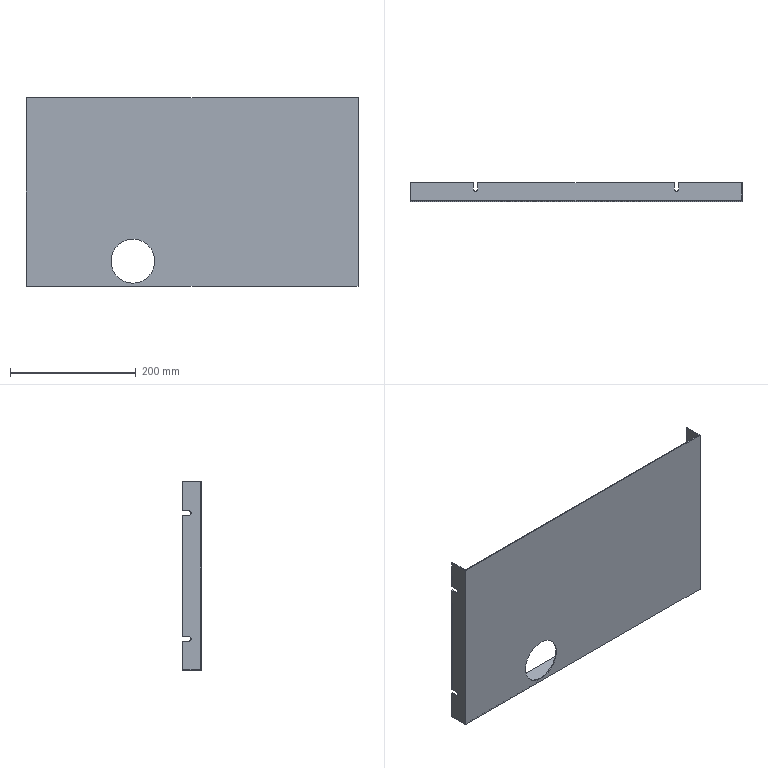Part | SolidWorks | features BaseBody 1 | 1 solid | 36 faces | box 528 x 30 x 300 mm | volume 279118 mm3 | plane 28 | cylinder 8 | commonest cylinder face diameters 7 x6 70 x2
STEP:
#1=CARTESIAN_POINT('',(-94.,1.5,-145.));
#2=VERTEX_POINT('',#1);
#3=CARTESIAN_POINT('',(-94.,1.5,-75.));
#4=VERTEX_POINT('',#3);
#5=CARTESIAN_POINT('',(-94.,1.5,-110.));
#6=DIRECTION('',(0.,1.,0.));
#7=DIRECTION('',(0.,0.,-1.));
#8=AXIS2_PLACEMENT_3D('',#5,#6,#7);
#9=CIRCLE('',#8,35.);
#10=EDGE_CURVE('',#2,#4,#9,.T.);
#11=ORIENTED_EDGE('',*,*,#10,.T.);
#12=CARTESIAN_POINT('',(-94.,0.,-75.));
#13=VERTEX_POINT('',#12);
#14=CARTESIAN_POINT('',(-94.,30.001,-75.));
#15=DIRECTION('',(0.,-1.,0.));
#16=VECTOR('',#15,1000.);
#17=LINE('',#14,#16);
#18=EDGE_CURVE('',#4,#13,#17,.T.);
#19=ORIENTED_EDGE('',*,*,#18,.T.);
#20=CARTESIAN_POINT('',(-94.,0.,-145.));
#21=VERTEX_POINT('',#20);
#22=CARTESIAN_POINT('',(-94.,0.,-110.));
#23=DIRECTION('',(0.,-1.,0.));
#24=DIRECTION('',(0.,0.,-1.));
#25=AXIS2_PLACEMENT_3D('',#22,#23,#24);
#26=CIRCLE('',#25,35.);
#27=EDGE_CURVE('',#13,#21,#26,.T.);
#28=ORIENTED_EDGE('',*,*,#27,.T.);
#29=CARTESIAN_POINT('',(-94.,30.001,-145.));
#30=DIRECTION('',(0.,-1.,0.));
#31=VECTOR('',#30,1000.);
#32=LINE('',#29,#31);
#33=EDGE_CURVE('',#2,#21,#32,.T.);
#34=ORIENTED_EDGE('',*,*,#33,.F.);
#35=EDGE_LOOP('',(#11,#19,#28,#34));
#36=FACE_OUTER_BOUND('',#35,.T.);
#37=CARTESIAN_POINT('',(-94.,30.001,-110.));
#38=DIRECTION('',(0.,-1.,0.));
#39=DIRECTION('',(0.,0.,-1.));
#40=AXIS2_PLACEMENT_3D('',#37,#38,#39);
#41=CYLINDRICAL_SURFACE('',#40,35.);
#42=ADVANCED_FACE('',(#36),#41,.F.);
#43=CARTESIAN_POINT('',(-163.5,20.,-148.5));
#44=VERTEX_POINT('',#43);
#45=CARTESIAN_POINT('',(-163.5,20.,-150.));
#46=VERTEX_POINT('',#45);
#47=CARTESIAN_POINT('',(-163.5,20.,150.001));
#48=DIRECTION('',(0.,0.,-1.));
#49=VECTOR('',#48,1000.);
#50=LINE('',#47,#49);
#51=EDGE_CURVE('',#44,#46,#50,.T.);
#52=ORIENTED_EDGE('',*,*,#51,.T.);
#53=CARTESIAN_POINT('',(-163.5,30.,-150.));
#54=VERTEX_POINT('',#53);
#55=CARTESIAN_POINT('',(-163.5,30.,-150.));
#56=DIRECTION('',(0.,1.,0.));
#57=VECTOR('',#56,1000.);
#58=LINE('',#55,#57);
#59=EDGE_CURVE('',#46,#54,#58,.T.);
#60=ORIENTED_EDGE('',*,*,#59,.T.);
#61=CARTESIAN_POINT('',(-163.5,30.,-148.5));
#62=VERTEX_POINT('',#61);
#63=CARTESIAN_POINT('',(-163.5,30.,150.001));
#64=DIRECTION('',(0.,0.,1.));
#65=VECTOR('',#64,1000.);
#66=LINE('',#63,#65);
#67=EDGE_CURVE('',#54,#62,#66,.T.);
#68=ORIENTED_EDGE('',*,*,#67,.T.);
#69=CARTESIAN_POINT('',(-163.5,30.,-148.5));
#70=DIRECTION('',(0.,1.,0.));
#71=VECTOR('',#70,1000.);
#72=LINE('',#69,#71);
#73=EDGE_CURVE('',#44,#62,#72,.T.);
#74=ORIENTED_EDGE('',*,*,#73,.F.);
#75=EDGE_LOOP('',(#52,#60,#68,#74));
#76=FACE_OUTER_BOUND('',#75,.T.);
#77=CARTESIAN_POINT('',(-163.5,30.,150.001));
#78=DIRECTION('',(-1.,0.,0.));
#79=DIRECTION('',(0.,0.,1.));
#80=AXIS2_PLACEMENT_3D('',#77,#78,#79);
#81=PLANE('',#80);
#82=ADVANCED_FACE('',(#76),#81,.F.);
#83=CARTESIAN_POINT('',(-156.5,20.,-148.5));
#84=VERTEX_POINT('',#83);
#85=CARTESIAN_POINT('',(-156.5,20.,-150.));
#86=VERTEX_POINT('',#85);
#87=CARTESIAN_POINT('',(-156.5,20.,150.001));
#88=DIRECTION('',(0.,0.,-1.));
#89=VECTOR('',#88,1000.);
#90=LINE('',#87,#89);
#91=EDGE_CURVE('',#84,#86,#90,.T.);
#92=ORIENTED_EDGE('',*,*,#91,.T.);
#93=CARTESIAN_POINT('',(-160.,20.,-150.));
#94=DIRECTION('',(0.,0.,-1.));
#95=DIRECTION('',(-1.,0.,0.));
#96=AXIS2_PLACEMENT_3D('',#93,#94,#95);
#97=CIRCLE('',#96,3.5);
#98=EDGE_CURVE('',#86,#46,#97,.T.);
#99=ORIENTED_EDGE('',*,*,#98,.T.);
#100=ORIENTED_EDGE('',*,*,#51,.F.);
#101=CARTESIAN_POINT('',(-160.,20.,-148.5));
#102=DIRECTION('',(0.,0.,-1.));
#103=DIRECTION('',(1.,0.,0.));
#104=AXIS2_PLACEMENT_3D('',#101,#102,#103);
#105=CIRCLE('',#104,3.5);
#106=EDGE_CURVE('',#84,#44,#105,.T.);
#107=ORIENTED_EDGE('',*,*,#106,.F.);
#108=EDGE_LOOP('',(#92,#99,#100,#107));
#109=FACE_OUTER_BOUND('',#108,.T.);
#110=CARTESIAN_POINT('',(-160.,20.,150.001));
#111=DIRECTION('',(0.,0.,-1.));
#112=DIRECTION('',(-1.,0.,0.));
#113=AXIS2_PLACEMENT_3D('',#110,#111,#112);
#114=CYLINDRICAL_SURFACE('',#113,3.5);
#115=ADVANCED_FACE('',(#109),#114,.F.);
#116=CARTESIAN_POINT('',(-156.5,30.,-148.5));
#117=VERTEX_POINT('',#116);
#118=CARTESIAN_POINT('',(-156.5,30.,-150.));
#119=VERTEX_POINT('',#118);
#120=CARTESIAN_POINT('',(-156.5,30.,150.001));
#121=DIRECTION('',(0.,0.,-1.));
#122=VECTOR('',#121,1000.);
#123=LINE('',#120,#122);
#124=EDGE_CURVE('',#117,#119,#123,.T.);
#125=ORIENTED_EDGE('',*,*,#124,.T.);
#126=CARTESIAN_POINT('',(-156.5,30.,-150.));
#127=DIRECTION('',(0.,-1.,0.));
#128=VECTOR('',#127,1000.);
#129=LINE('',#126,#128);
#130=EDGE_CURVE('',#119,#86,#129,.T.);
#131=ORIENTED_EDGE('',*,*,#130,.T.);
#132=ORIENTED_EDGE('',*,*,#91,.F.);
#133=CARTESIAN_POINT('',(-156.5,30.,-148.5));
#134=DIRECTION('',(0.,-1.,0.));
#135=VECTOR('',#134,1000.);
#136=LINE('',#133,#135);
#137=EDGE_CURVE('',#117,#84,#136,.T.);
#138=ORIENTED_EDGE('',*,*,#137,.F.);
#139=EDGE_LOOP('',(#125,#131,#132,#138));
#140=FACE_OUTER_BOUND('',#139,.T.);
#141=CARTESIAN_POINT('',(-156.5,30.,150.001));
#142=DIRECTION('',(1.,0.,0.));
#143=DIRECTION('',(0.,1.,0.));
#144=AXIS2_PLACEMENT_3D('',#141,#142,#143);
#145=PLANE('',#144);
#146=ADVANCED_FACE('',(#140),#145,.F.);
#147=CARTESIAN_POINT('',(156.5,20.,-148.5));
#148=VERTEX_POINT('',#147);
#149=CARTESIAN_POINT('',(156.5,20.,-150.));
#150=VERTEX_POINT('',#149);
#151=CARTESIAN_POINT('',(156.5,20.,150.001));
#152=DIRECTION('',(0.,0.,-1.));
#153=VECTOR('',#152,1000.);
#154=LINE('',#151,#153);
#155=EDGE_CURVE('',#148,#150,#154,.T.);
#156=ORIENTED_EDGE('',*,*,#155,.T.);
#157=CARTESIAN_POINT('',(156.5,30.,-150.));
#158=VERTEX_POINT('',#157);
#159=CARTESIAN_POINT('',(156.5,30.,-150.));
#160=DIRECTION('',(0.,1.,0.));
#161=VECTOR('',#160,1000.);
#162=LINE('',#159,#161);
#163=EDGE_CURVE('',#150,#158,#162,.T.);
#164=ORIENTED_EDGE('',*,*,#163,.T.);
#165=CARTESIAN_POINT('',(156.5,30.,-148.5));
#166=VERTEX_POINT('',#165);
#167=CARTESIAN_POINT('',(156.5,30.,150.001));
#168=DIRECTION('',(0.,0.,1.));
#169=VECTOR('',#168,1000.);
#170=LINE('',#167,#169);
#171=EDGE_CURVE('',#158,#166,#170,.T.);
#172=ORIENTED_EDGE('',*,*,#171,.T.);
#173=CARTESIAN_POINT('',(156.5,30.,-148.5));
#174=DIRECTION('',(0.,1.,0.));
#175=VECTOR('',#174,1000.);
#176=LINE('',#173,#175);
#177=EDGE_CURVE('',#148,#166,#176,.T.);
#178=ORIENTED_EDGE('',*,*,#177,.F.);
#179=EDGE_LOOP('',(#156,#164,#172,#178));
#180=FACE_OUTER_BOUND('',#179,.T.);
#181=CARTESIAN_POINT('',(156.5,30.,150.001));
#182=DIRECTION('',(-1.,0.,0.));
#183=DIRECTION('',(0.,0.,1.));
#184=AXIS2_PLACEMENT_3D('',#181,#182,#183);
#185=PLANE('',#184);
#186=ADVANCED_FACE('',(#180),#185,.F.);
#187=CARTESIAN_POINT('',(163.5,20.,-148.5));
#188=VERTEX_POINT('',#187);
#189=CARTESIAN_POINT('',(163.5,20.,-150.));
#190=VERTEX_POINT('',#189);
#191=CARTESIAN_POINT('',(163.5,20.,150.001));
#192=DIRECTION('',(0.,0.,-1.));
#193=VECTOR('',#192,1000.);
#194=LINE('',#191,#193);
#195=EDGE_CURVE('',#188,#190,#194,.T.);
#196=ORIENTED_EDGE('',*,*,#195,.T.);
#197=CARTESIAN_POINT('',(160.,20.,-150.));
#198=DIRECTION('',(0.,0.,-1.));
#199=DIRECTION('',(-1.,0.,0.));
#200=AXIS2_PLACEMENT_3D('',#197,#198,#199);
#201=CIRCLE('',#200,3.5);
#202=EDGE_CURVE('',#190,#150,#201,.T.);
#203=ORIENTED_EDGE('',*,*,#202,.T.);
#204=ORIENTED_EDGE('',*,*,#155,.F.);
#205=CARTESIAN_POINT('',(160.,20.,-148.5));
#206=DIRECTION('',(0.,0.,-1.));
#207=DIRECTION('',(1.,0.,0.));
#208=AXIS2_PLACEMENT_3D('',#205,#206,#207);
#209=CIRCLE('',#208,3.5);
#210=EDGE_CURVE('',#188,#148,#209,.T.);
#211=ORIENTED_EDGE('',*,*,#210,.F.);
#212=EDGE_LOOP('',(#196,#203,#204,#211));
#213=FACE_OUTER_BOUND('',#212,.T.);
#214=CARTESIAN_POINT('',(160.,20.,150.001));
#215=DIRECTION('',(0.,0.,-1.));
#216=DIRECTION('',(-1.,0.,0.));
#217=AXIS2_PLACEMENT_3D('',#214,#215,#216);
#218=CYLINDRICAL_SURFACE('',#217,3.5);
#219=ADVANCED_FACE('',(#213),#218,.F.);
#220=CARTESIAN_POINT('',(163.5,30.,-148.5));
#221=VERTEX_POINT('',#220);
#222=CARTESIAN_POINT('',(163.5,30.,-150.));
#223=VERTEX_POINT('',#222);
#224=CARTESIAN_POINT('',(163.5,30.,150.001));
#225=DIRECTION('',(0.,0.,-1.));
#226=VECTOR('',#225,1000.);
#227=LINE('',#224,#226);
#228=EDGE_CURVE('',#221,#223,#227,.T.);
#229=ORIENTED_EDGE('',*,*,#228,.T.);
#230=CARTESIAN_POINT('',(163.5,30.,-150.));
#231=DIRECTION('',(0.,-1.,0.));
#232=VECTOR('',#231,1000.);
#233=LINE('',#230,#232);
#234=EDGE_CURVE('',#223,#190,#233,.T.);
#235=ORIENTED_EDGE('',*,*,#234,.T.);
#236=ORIENTED_EDGE('',*,*,#195,.F.);
#237=CARTESIAN_POINT('',(163.5,30.,-148.5));
#238=DIRECTION('',(0.,-1.,0.));
#239=VECTOR('',#238,1000.);
#240=LINE('',#237,#239);
#241=EDGE_CURVE('',#221,#188,#240,.T.);
#242=ORIENTED_EDGE('',*,*,#241,.F.);
#243=EDGE_LOOP('',(#229,#235,#236,#242));
#244=FACE_OUTER_BOUND('',#243,.T.);
#245=CARTESIAN_POINT('',(163.5,30.,150.001));
#246=DIRECTION('',(1.,0.,0.));
#247=DIRECTION('',(0.,1.,0.));
#248=AXIS2_PLACEMENT_3D('',#245,#246,#247);
#249=PLANE('',#248);
#250=ADVANCED_FACE('',(#244),#249,.F.);
#251=CARTESIAN_POINT('',(262.5,20.,-96.5));
#252=VERTEX_POINT('',#251);
#253=CARTESIAN_POINT('',(262.5,30.,-96.5));
#254=VERTEX_POINT('',#253);
#255=CARTESIAN_POINT('',(262.5,30.,-96.5));
#256=DIRECTION('',(0.,1.,0.));
#257=VECTOR('',#256,1000.);
#258=LINE('',#255,#257);
#259=EDGE_CURVE('',#252,#254,#258,.T.);
#260=ORIENTED_EDGE('',*,*,#259,.T.);
#261=CARTESIAN_POINT('',(264.,30.,-96.5));
#262=VERTEX_POINT('',#261);
#263=CARTESIAN_POINT('',(-264.,30.,-96.5));
#264=DIRECTION('',(1.,0.,0.));
#265=VECTOR('',#264,1000.);
#266=LINE('',#263,#265);
#267=EDGE_CURVE('',#254,#262,#266,.T.);
#268=ORIENTED_EDGE('',*,*,#267,.T.);
#269=CARTESIAN_POINT('',(264.,20.,-96.5));
#270=VERTEX_POINT('',#269);
#271=CARTESIAN_POINT('',(264.,30.,-96.5));
#272=DIRECTION('',(0.,-1.,0.));
#273=VECTOR('',#272,1000.);
#274=LINE('',#271,#273);
#275=EDGE_CURVE('',#262,#270,#274,.T.);
#276=ORIENTED_EDGE('',*,*,#275,.T.);
#277=CARTESIAN_POINT('',(-264.,20.,-96.5));
#278=DIRECTION('',(1.,0.,0.));
#279=VECTOR('',#278,1000.);
#280=LINE('',#277,#279);
#281=EDGE_CURVE('',#252,#270,#280,.T.);
#282=ORIENTED_EDGE('',*,*,#281,.F.);
#283=EDGE_LOOP('',(#260,#268,#276,#282));
#284=FACE_OUTER_BOUND('',#283,.T.);
#285=CARTESIAN_POINT('',(-264.,30.,-96.5));
#286=DIRECTION('',(0.,0.,1.));
#287=DIRECTION('',(1.,0.,0.));
#288=AXIS2_PLACEMENT_3D('',#285,#286,#287);
#289=PLANE('',#288);
#290=ADVANCED_FACE('',(#284),#289,.F.);
#291=CARTESIAN_POINT('',(262.5,20.,-103.5));
#292=VERTEX_POINT('',#291);
#293=CARTESIAN_POINT('',(262.5,20.,-100.));
#294=DIRECTION('',(-1.,0.,0.));
#295=DIRECTION('',(0.,0.,1.));
#296=AXIS2_PLACEMENT_3D('',#293,#294,#295);
#297=CIRCLE('',#296,3.5);
#298=EDGE_CURVE('',#292,#252,#297,.T.);
#299=ORIENTED_EDGE('',*,*,#298,.T.);
#300=ORIENTED_EDGE('',*,*,#281,.T.);
#301=CARTESIAN_POINT('',(264.,20.,-103.5));
#302=VERTEX_POINT('',#301);
#303=CARTESIAN_POINT('',(264.,20.,-100.));
#304=DIRECTION('',(1.,0.,0.));
#305=DIRECTION('',(0.,0.,1.));
#306=AXIS2_PLACEMENT_3D('',#303,#304,#305);
#307=CIRCLE('',#306,3.5);
#308=EDGE_CURVE('',#270,#302,#307,.T.);
#309=ORIENTED_EDGE('',*,*,#308,.T.);
#310=CARTESIAN_POINT('',(-264.,20.,-103.5));
#311=DIRECTION('',(1.,0.,0.));
#312=VECTOR('',#311,1000.);
#313=LINE('',#310,#312);
#314=EDGE_CURVE('',#292,#302,#313,.T.);
#315=ORIENTED_EDGE('',*,*,#314,.F.);
#316=EDGE_LOOP('',(#299,#300,#309,#315));
#317=FACE_OUTER_BOUND('',#316,.T.);
#318=CARTESIAN_POINT('',(-264.,20.,-100.));
#319=DIRECTION('',(1.,0.,0.));
#320=DIRECTION('',(0.,0.,-1.));
#321=AXIS2_PLACEMENT_3D('',#318,#319,#320);
#322=CYLINDRICAL_SURFACE('',#321,3.5);
#323=ADVANCED_FACE('',(#317),#322,.F.);
#324=CARTESIAN_POINT('',(262.5,30.,-103.5));
#325=VERTEX_POINT('',#324);
#326=CARTESIAN_POINT('',(262.5,30.,-103.5));
#327=DIRECTION('',(0.,-1.,0.));
#328=VECTOR('',#327,1000.);
#329=LINE('',#326,#328);
#330=EDGE_CURVE('',#325,#292,#329,.T.);
#331=ORIENTED_EDGE('',*,*,#330,.T.);
#332=ORIENTED_EDGE('',*,*,#314,.T.);
#333=CARTESIAN_POINT('',(264.,30.,-103.5));
#334=VERTEX_POINT('',#333);
#335=CARTESIAN_POINT('',(264.,30.,-103.5));
#336=DIRECTION('',(0.,1.,0.));
#337=VECTOR('',#336,1000.);
#338=LINE('',#335,#337);
#339=EDGE_CURVE('',#302,#334,#338,.T.);
#340=ORIENTED_EDGE('',*,*,#339,.T.);
#341=CARTESIAN_POINT('',(-264.,30.,-103.5));
#342=DIRECTION('',(1.,0.,0.));
#343=VECTOR('',#342,1000.);
#344=LINE('',#341,#343);
#345=EDGE_CURVE('',#325,#334,#344,.T.);
#346=ORIENTED_EDGE('',*,*,#345,.F.);
#347=EDGE_LOOP('',(#331,#332,#340,#346));
#348=FACE_OUTER_BOUND('',#347,.T.);
#349=CARTESIAN_POINT('',(-264.,30.,-103.5));
#350=DIRECTION('',(0.,0.,-1.));
#351=DIRECTION('',(0.,-1.,0.));
#352=AXIS2_PLACEMENT_3D('',#349,#350,#351);
#353=PLANE('',#352);
#354=ADVANCED_FACE('',(#348),#353,.F.);
#355=CARTESIAN_POINT('',(-262.5,20.,-103.5));
#356=VERTEX_POINT('',#355);
#357=CARTESIAN_POINT('',(-262.5,30.,-103.5));
#358=VERTEX_POINT('',#357);
#359=CARTESIAN_POINT('',(-262.5,30.,-103.5));
#360=DIRECTION('',(0.,1.,0.));
#361=VECTOR('',#360,1000.);
#362=LINE('',#359,#361);
#363=EDGE_CURVE('',#356,#358,#362,.T.);
#364=ORIENTED_EDGE('',*,*,#363,.T.);
#365=CARTESIAN_POINT('',(-264.,30.,-103.5));
#366=VERTEX_POINT('',#365);
#367=CARTESIAN_POINT('',(-264.,30.,-103.5));
#368=DIRECTION('',(1.,0.,0.));
#369=VECTOR('',#368,1000.);
#370=LINE('',#367,#369);
#371=EDGE_CURVE('',#366,#358,#370,.T.);
#372=ORIENTED_EDGE('',*,*,#371,.F.);
#373=CARTESIAN_POINT('',(-264.,20.,-103.5));
#374=VERTEX_POINT('',#373);
#375=CARTESIAN_POINT('',(-264.,30.,-103.5));
#376=DIRECTION('',(0.,1.,0.));
#377=VECTOR('',#376,1000.);
#378=LINE('',#375,#377);
#379=EDGE_CURVE('',#374,#366,#378,.T.);
#380=ORIENTED_EDGE('',*,*,#379,.F.);
#381=CARTESIAN_POINT('',(-264.,20.,-103.5));
#382=DIRECTION('',(1.,0.,0.));
#383=VECTOR('',#382,1000.);
#384=LINE('',#381,#383);
#385=EDGE_CURVE('',#374,#356,#384,.T.);
#386=ORIENTED_EDGE('',*,*,#385,.T.);
#387=EDGE_LOOP('',(#364,#372,#380,#386));
#388=FACE_OUTER_BOUND('',#387,.T.);
#389=CARTESIAN_POINT('',(-264.,30.,-103.5));
#390=DIRECTION('',(0.,0.,-1.));
#391=DIRECTION('',(0.,-1.,0.));
#392=AXIS2_PLACEMENT_3D('',#389,#390,#391);
#393=PLANE('',#392);
#394=ADVANCED_FACE('',(#388),#393,.F.);
#395=CARTESIAN_POINT('',(-262.5,20.,-96.5));
#396=VERTEX_POINT('',#395);
#397=CARTESIAN_POINT('',(-262.5,20.,-100.));
#398=DIRECTION('',(1.,0.,0.));
#399=DIRECTION('',(0.,0.,-1.));
#400=AXIS2_PLACEMENT_3D('',#397,#398,#399);
#401=CIRCLE('',#400,3.5);
#402=EDGE_CURVE('',#396,#356,#401,.T.);
#403=ORIENTED_EDGE('',*,*,#402,.T.);
#404=ORIENTED_EDGE('',*,*,#385,.F.);
#405=CARTESIAN_POINT('',(-264.,20.,-96.5));
#406=VERTEX_POINT('',#405);
#407=CARTESIAN_POINT('',(-264.,20.,-100.));
#408=DIRECTION('',(1.,0.,0.));
#409=DIRECTION('',(0.,0.,1.));
#410=AXIS2_PLACEMENT_3D('',#407,#408,#409);
#411=CIRCLE('',#410,3.5);
#412=EDGE_CURVE('',#406,#374,#411,.T.);
#413=ORIENTED_EDGE('',*,*,#412,.F.);
#414=CARTESIAN_POINT('',(-264.,20.,-96.5));
#415=DIRECTION('',(1.,0.,0.));
#416=VECTOR('',#415,1000.);
#417=LINE('',#414,#416);
#418=EDGE_CURVE('',#406,#396,#417,.T.);
#419=ORIENTED_EDGE('',*,*,#418,.T.);
#420=EDGE_LOOP('',(#403,#404,#413,#419));
#421=FACE_OUTER_BOUND('',#420,.T.);
#422=CARTESIAN_POINT('',(-264.,20.,-100.));
#423=DIRECTION('',(1.,0.,0.));
#424=DIRECTION('',(0.,0.,-1.));
#425=AXIS2_PLACEMENT_3D('',#422,#423,#424);
#426=CYLINDRICAL_SURFACE('',#425,3.5);
#427=ADVANCED_FACE('',(#421),#426,.F.);
#428=CARTESIAN_POINT('',(-262.5,30.,-96.5));
#429=VERTEX_POINT('',#428);
#430=CARTESIAN_POINT('',(-262.5,30.,-96.5));
#431=DIRECTION('',(0.,-1.,0.));
#432=VECTOR('',#431,1000.);
#433=LINE('',#430,#432);
#434=EDGE_CURVE('',#429,#396,#433,.T.);
#435=ORIENTED_EDGE('',*,*,#434,.T.);
#436=ORIENTED_EDGE('',*,*,#418,.F.);
#437=CARTESIAN_POINT('',(-264.,30.,-96.5));
#438=VERTEX_POINT('',#437);
#439=CARTESIAN_POINT('',(-264.,30.,-96.5));
#440=DIRECTION('',(0.,-1.,0.));
#441=VECTOR('',#440,1000.);
#442=LINE('',#439,#441);
#443=EDGE_CURVE('',#438,#406,#442,.T.);
#444=ORIENTED_EDGE('',*,*,#443,.F.);
#445=CARTESIAN_POINT('',(-264.,30.,-96.5));
#446=DIRECTION('',(1.,0.,0.));
#447=VECTOR('',#446,1000.);
#448=LINE('',#445,#447);
#449=EDGE_CURVE('',#438,#429,#448,.T.);
#450=ORIENTED_EDGE('',*,*,#449,.T.);
#451=EDGE_LOOP('',(#435,#436,#444,#450));
#452=FACE_OUTER_BOUND('',#451,.T.);
#453=CARTESIAN_POINT('',(-264.,30.,-96.5));
#454=DIRECTION('',(0.,0.,1.));
#455=DIRECTION('',(1.,0.,0.));
#456=AXIS2_PLACEMENT_3D('',#453,#454,#455);
#457=PLANE('',#456);
#458=ADVANCED_FACE('',(#452),#457,.F.);
#459=CARTESIAN_POINT('',(262.5,20.,103.5));
#460=VERTEX_POINT('',#459);
#461=CARTESIAN_POINT('',(262.5,30.,103.5));
#462=VERTEX_POINT('',#461);
#463=CARTESIAN_POINT('',(262.5,30.,103.5));
#464=DIRECTION('',(0.,1.,0.));
#465=VECTOR('',#464,1000.);
#466=LINE('',#463,#465);
#467=EDGE_CURVE('',#460,#462,#466,.T.);
#468=ORIENTED_EDGE('',*,*,#467,.T.);
#469=CARTESIAN_POINT('',(264.,30.,103.5));
#470=VERTEX_POINT('',#469);
#471=CARTESIAN_POINT('',(-264.,30.,103.5));
#472=DIRECTION('',(1.,0.,0.));
#473=VECTOR('',#472,1000.);
#474=LINE('',#471,#473);
#475=EDGE_CURVE('',#462,#470,#474,.T.);
#476=ORIENTED_EDGE('',*,*,#475,.T.);
#477=CARTESIAN_POINT('',(264.,20.,103.5));
#478=VERTEX_POINT('',#477);
#479=CARTESIAN_POINT('',(264.,30.,103.5));
#480=DIRECTION('',(0.,-1.,0.));
#481=VECTOR('',#480,1000.);
#482=LINE('',#479,#481);
#483=EDGE_CURVE('',#470,#478,#482,.T.);
#484=ORIENTED_EDGE('',*,*,#483,.T.);
#485=CARTESIAN_POINT('',(-264.,20.,103.5));
#486=DIRECTION('',(1.,0.,0.));
#487=VECTOR('',#486,1000.);
#488=LINE('',#485,#487);
#489=EDGE_CURVE('',#460,#478,#488,.T.);
#490=ORIENTED_EDGE('',*,*,#489,.F.);
#491=EDGE_LOOP('',(#468,#476,#484,#490));
#492=FACE_OUTER_BOUND('',#491,.T.);
#493=CARTESIAN_POINT('',(-264.,30.,103.5));
#494=DIRECTION('',(0.,0.,1.));
#495=DIRECTION('',(1.,0.,0.));
#496=AXIS2_PLACEMENT_3D('',#493,#494,#495);
#497=PLANE('',#496);
#498=ADVANCED_FACE('',(#492),#497,.F.);
#499=CARTESIAN_POINT('',(262.5,20.,96.5));
#500=VERTEX_POINT('',#499);
#501=CARTESIAN_POINT('',(262.5,20.,100.));
#502=DIRECTION('',(-1.,0.,0.));
#503=DIRECTION('',(0.,0.,1.));
#504=AXIS2_PLACEMENT_3D('',#501,#502,#503);
#505=CIRCLE('',#504,3.5);
#506=EDGE_CURVE('',#500,#460,#505,.T.);
#507=ORIENTED_EDGE('',*,*,#506,.T.);
#508=ORIENTED_EDGE('',*,*,#489,.T.);
#509=CARTESIAN_POINT('',(264.,20.,96.5));
#510=VERTEX_POINT('',#509);
#511=CARTESIAN_POINT('',(264.,20.,100.));
#512=DIRECTION('',(1.,0.,0.));
#513=DIRECTION('',(0.,0.,-1.));
#514=AXIS2_PLACEMENT_3D('',#511,#512,#513);
#515=CIRCLE('',#514,3.5);
#516=EDGE_CURVE('',#478,#510,#515,.T.);
#517=ORIENTED_EDGE('',*,*,#516,.T.);
#518=CARTESIAN_POINT('',(-264.,20.,96.5));
#519=DIRECTION('',(1.,0.,0.));
#520=VECTOR('',#519,1000.);
#521=LINE('',#518,#520);
#522=EDGE_CURVE('',#500,#510,#521,.T.);
#523=ORIENTED_EDGE('',*,*,#522,.F.);
#524=EDGE_LOOP('',(#507,#508,#517,#523));
#525=FACE_OUTER_BOUND('',#524,.T.);
#526=CARTESIAN_POINT('',(-264.,20.,100.));
#527=DIRECTION('',(1.,0.,0.));
#528=DIRECTION('',(0.,0.,-1.));
#529=AXIS2_PLACEMENT_3D('',#526,#527,#528);
#530=CYLINDRICAL_SURFACE('',#529,3.5);
#531=ADVANCED_FACE('',(#525),#530,.F.);
#532=CARTESIAN_POINT('',(262.5,30.,96.5));
#533=VERTEX_POINT('',#532);
#534=CARTESIAN_POINT('',(262.5,30.,96.5));
#535=DIRECTION('',(0.,-1.,0.));
#536=VECTOR('',#535,1000.);
#537=LINE('',#534,#536);
#538=EDGE_CURVE('',#533,#500,#537,.T.);
#539=ORIENTED_EDGE('',*,*,#538,.T.);
#540=ORIENTED_EDGE('',*,*,#522,.T.);
#541=CARTESIAN_POINT('',(264.,30.,96.5));
#542=VERTEX_POINT('',#541);
#543=CARTESIAN_POINT('',(264.,30.,96.5));
#544=DIRECTION('',(0.,1.,0.));
#545=VECTOR('',#544,1000.);
#546=LINE('',#543,#545);
#547=EDGE_CURVE('',#510,#542,#546,.T.);
#548=ORIENTED_EDGE('',*,*,#547,.T.);
#549=CARTESIAN_POINT('',(-264.,30.,96.5));
#550=DIRECTION('',(1.,0.,0.));
#551=VECTOR('',#550,1000.);
#552=LINE('',#549,#551);
#553=EDGE_CURVE('',#533,#542,#552,.T.);
#554=ORIENTED_EDGE('',*,*,#553,.F.);
#555=EDGE_LOOP('',(#539,#540,#548,#554));
#556=FACE_OUTER_BOUND('',#555,.T.);
#557=CARTESIAN_POINT('',(-264.,30.,96.5));
#558=DIRECTION('',(0.,0.,-1.));
#559=DIRECTION('',(0.,-1.,0.));
#560=AXIS2_PLACEMENT_3D('',#557,#558,#559);
#561=PLANE('',#560);
#562=ADVANCED_FACE('',(#556),#561,.F.);
#563=CARTESIAN_POINT('',(-262.5,20.,96.5));
#564=VERTEX_POINT('',#563);
#565=CARTESIAN_POINT('',(-262.5,30.,96.5));
#566=VERTEX_POINT('',#565);
#567=CARTESIAN_POINT('',(-262.5,30.,96.5));
#568=DIRECTION('',(0.,1.,0.));
#569=VECTOR('',#568,1000.);
#570=LINE('',#567,#569);
#571=EDGE_CURVE('',#564,#566,#570,.T.);
#572=ORIENTED_EDGE('',*,*,#571,.T.);
#573=CARTESIAN_POINT('',(-264.,30.,96.5));
#574=VERTEX_POINT('',#573);
#575=CARTESIAN_POINT('',(-264.,30.,96.5));
#576=DIRECTION('',(1.,0.,0.));
#577=VECTOR('',#576,1000.);
#578=LINE('',#575,#577);
#579=EDGE_CURVE('',#574,#566,#578,.T.);
#580=ORIENTED_EDGE('',*,*,#579,.F.);
#581=CARTESIAN_POINT('',(-264.,20.,96.5));
#582=VERTEX_POINT('',#581);
#583=CARTESIAN_POINT('',(-264.,30.,96.5));
#584=DIRECTION('',(0.,1.,0.));
#585=VECTOR('',#584,1000.);
#586=LINE('',#583,#585);
#587=EDGE_CURVE('',#582,#574,#586,.T.);
#588=ORIENTED_EDGE('',*,*,#587,.F.);
#589=CARTESIAN_POINT('',(-264.,20.,96.5));
#590=DIRECTION('',(1.,0.,0.));
#591=VECTOR('',#590,1000.);
#592=LINE('',#589,#591);
#593=EDGE_CURVE('',#582,#564,#592,.T.);
#594=ORIENTED_EDGE('',*,*,#593,.T.);
#595=EDGE_LOOP('',(#572,#580,#588,#594));
#596=FACE_OUTER_BOUND('',#595,.T.);
#597=CARTESIAN_POINT('',(-264.,30.,96.5));
#598=DIRECTION('',(0.,0.,-1.));
#599=DIRECTION('',(0.,-1.,0.));
#600=AXIS2_PLACEMENT_3D('',#597,#598,#599);
#601=PLANE('',#600);
#602=ADVANCED_FACE('',(#596),#601,.F.);
#603=CARTESIAN_POINT('',(-262.5,20.,103.5));
#604=VERTEX_POINT('',#603);
#605=CARTESIAN_POINT('',(-262.5,20.,100.));
#606=DIRECTION('',(1.,0.,0.));
#607=DIRECTION('',(0.,0.,-1.));
#608=AXIS2_PLACEMENT_3D('',#605,#606,#607);
#609=CIRCLE('',#608,3.5);
#610=EDGE_CURVE('',#604,#564,#609,.T.);
#611=ORIENTED_EDGE('',*,*,#610,.T.);
#612=ORIENTED_EDGE('',*,*,#593,.F.);
#613=CARTESIAN_POINT('',(-264.,20.,103.5));
#614=VERTEX_POINT('',#613);
#615=CARTESIAN_POINT('',(-264.,20.,100.));
#616=DIRECTION('',(1.,0.,0.));
#617=DIRECTION('',(0.,0.,-1.));
#618=AXIS2_PLACEMENT_3D('',#615,#616,#617);
#619=CIRCLE('',#618,3.5);
#620=EDGE_CURVE('',#614,#582,#619,.T.);
#621=ORIENTED_EDGE('',*,*,#620,.F.);
#622=CARTESIAN_POINT('',(-264.,20.,103.5));
#623=DIRECTION('',(1.,0.,0.));
#624=VECTOR('',#623,1000.);
#625=LINE('',#622,#624);
#626=EDGE_CURVE('',#614,#604,#625,.T.);
#627=ORIENTED_EDGE('',*,*,#626,.T.);
#628=EDGE_LOOP('',(#611,#612,#621,#627));
#629=FACE_OUTER_BOUND('',#628,.T.);
#630=CARTESIAN_POINT('',(-264.,20.,100.));
#631=DIRECTION('',(1.,0.,0.));
#632=DIRECTION('',(0.,0.,-1.));
#633=AXIS2_PLACEMENT_3D('',#630,#631,#632);
#634=CYLINDRICAL_SURFACE('',#633,3.5);
#635=ADVANCED_FACE('',(#629),#634,.F.);
#636=CARTESIAN_POINT('',(-262.5,30.,103.5));
#637=VERTEX_POINT('',#636);
#638=CARTESIAN_POINT('',(-262.5,30.,103.5));
#639=DIRECTION('',(0.,-1.,0.));
#640=VECTOR('',#639,1000.);
#641=LINE('',#638,#640);
#642=EDGE_CURVE('',#637,#604,#641,.T.);
#643=ORIENTED_EDGE('',*,*,#642,.T.);
#644=ORIENTED_EDGE('',*,*,#626,.F.);
#645=CARTESIAN_POINT('',(-264.,30.,103.5));
#646=VERTEX_POINT('',#645);
#647=CARTESIAN_POINT('',(-264.,30.,103.5));
#648=DIRECTION('',(0.,-1.,0.));
#649=VECTOR('',#648,1000.);
#650=LINE('',#647,#649);
#651=EDGE_CURVE('',#646,#614,#650,.T.);
#652=ORIENTED_EDGE('',*,*,#651,.F.);
#653=CARTESIAN_POINT('',(-264.,30.,103.5));
#654=DIRECTION('',(1.,0.,0.));
#655=VECTOR('',#654,1000.);
#656=LINE('',#653,#655);
#657=EDGE_CURVE('',#646,#637,#656,.T.);
#658=ORIENTED_EDGE('',*,*,#657,.T.);
#659=EDGE_LOOP('',(#643,#644,#652,#658));
#660=FACE_OUTER_BOUND('',#659,.T.);
#661=CARTESIAN_POINT('',(-264.,30.,103.5));
#662=DIRECTION('',(0.,0.,1.));
#663=DIRECTION('',(1.,0.,0.));
#664=AXIS2_PLACEMENT_3D('',#661,#662,#663);
#665=PLANE('',#664);
#666=ADVANCED_FACE('',(#660),#665,.F.);
#667=ORIENTED_EDGE('',*,*,#10,.F.);
#668=CARTESIAN_POINT('',(-94.,1.5,-110.));
#669=DIRECTION('',(0.,1.,0.));
#670=DIRECTION('',(0.,0.,-1.));
#671=AXIS2_PLACEMENT_3D('',#668,#669,#670);
#672=CIRCLE('',#671,35.);
#673=EDGE_CURVE('',#4,#2,#672,.T.);
#674=ORIENTED_EDGE('',*,*,#673,.F.);
#675=EDGE_LOOP('',(#667,#674));
#676=FACE_BOUND('',#675,.T.);
#677=CARTESIAN_POINT('',(262.5,1.5,150.));
#678=VERTEX_POINT('',#677);
#679=CARTESIAN_POINT('',(262.5,1.5,-148.5));
#680=VERTEX_POINT('',#679);
#681=CARTESIAN_POINT('',(262.5,1.5,0.));
#682=DIRECTION('',(0.,0.,-1.));
#683=VECTOR('',#682,1000.);
#684=LINE('',#681,#683);
#685=EDGE_CURVE('',#678,#680,#684,.T.);
#686=ORIENTED_EDGE('',*,*,#685,.T.);
#687=CARTESIAN_POINT('',(-262.5,1.5,-148.5));
#688=VERTEX_POINT('',#687);
#689=CARTESIAN_POINT('',(0.,1.5,-148.5));
#690=DIRECTION('',(-1.,0.,0.));
#691=VECTOR('',#690,1000.);
#692=LINE('',#689,#691);
#693=EDGE_CURVE('',#680,#688,#692,.T.);
#694=ORIENTED_EDGE('',*,*,#693,.T.);
#695=CARTESIAN_POINT('',(-262.5,1.5,150.));
#696=VERTEX_POINT('',#695);
#697=CARTESIAN_POINT('',(-262.5,1.5,0.));
#698=DIRECTION('',(0.,0.,1.));
#699=VECTOR('',#698,1000.);
#700=LINE('',#697,#699);
#701=EDGE_CURVE('',#688,#696,#700,.T.);
#702=ORIENTED_EDGE('',*,*,#701,.T.);
#703=CARTESIAN_POINT('',(-262.5,1.5,150.));
#704=DIRECTION('',(1.,0.,0.));
#705=VECTOR('',#704,1000.);
#706=LINE('',#703,#705);
#707=EDGE_CURVE('',#696,#678,#706,.T.);
#708=ORIENTED_EDGE('',*,*,#707,.T.);
#709=EDGE_LOOP('',(#686,#694,#702,#708));
#710=FACE_OUTER_BOUND('',#709,.T.);
#711=CARTESIAN_POINT('',(0.,1.5,0.));
#712=DIRECTION('',(0.,-1.,0.));
#713=DIRECTION('',(0.,0.,-1.));
#714=AXIS2_PLACEMENT_3D('',#711,#712,#713);
#715=PLANE('',#714);
#716=ADVANCED_FACE('',(#676,#710),#715,.F.);
#717=ORIENTED_EDGE('',*,*,#363,.F.);
#718=ORIENTED_EDGE('',*,*,#402,.F.);
#719=ORIENTED_EDGE('',*,*,#434,.F.);
#720=CARTESIAN_POINT('',(-262.5,30.,0.));
#721=DIRECTION('',(0.,0.,1.));
#722=VECTOR('',#721,1000.);
#723=LINE('',#720,#722);
#724=EDGE_CURVE('',#429,#566,#723,.T.);
#725=ORIENTED_EDGE('',*,*,#724,.T.);
#726=ORIENTED_EDGE('',*,*,#571,.F.);
#727=ORIENTED_EDGE('',*,*,#610,.F.);
#728=ORIENTED_EDGE('',*,*,#642,.F.);
#729=CARTESIAN_POINT('',(-262.5,30.,150.));
#730=VERTEX_POINT('',#729);
#731=CARTESIAN_POINT('',(-262.5,30.,0.));
#732=DIRECTION('',(0.,0.,1.));
#733=VECTOR('',#732,1000.);
#734=LINE('',#731,#733);
#735=EDGE_CURVE('',#637,#730,#734,.T.);
#736=ORIENTED_EDGE('',*,*,#735,.T.);
#737=CARTESIAN_POINT('',(-262.5,-523.502,150.));
#738=DIRECTION('',(0.,1.,0.));
#739=VECTOR('',#738,1000.);
#740=LINE('',#737,#739);
#741=EDGE_CURVE('',#696,#730,#740,.T.);
#742=ORIENTED_EDGE('',*,*,#741,.F.);
#743=ORIENTED_EDGE('',*,*,#701,.F.);
#744=CARTESIAN_POINT('',(-262.5,30.,-148.5));
#745=VERTEX_POINT('',#744);
#746=CARTESIAN_POINT('',(-262.5,30.,-148.5));
#747=DIRECTION('',(0.,-1.,0.));
#748=VECTOR('',#747,1000.);
#749=LINE('',#746,#748);
#750=EDGE_CURVE('',#745,#688,#749,.T.);
#751=ORIENTED_EDGE('',*,*,#750,.F.);
#752=CARTESIAN_POINT('',(-262.5,30.,0.));
#753=DIRECTION('',(0.,0.,1.));
#754=VECTOR('',#753,1000.);
#755=LINE('',#752,#754);
#756=EDGE_CURVE('',#745,#358,#755,.T.);
#757=ORIENTED_EDGE('',*,*,#756,.T.);
#758=EDGE_LOOP('',(#717,#718,#719,#725,#726,#727,#728,#736,#742,#743,#751,#757));
#759=FACE_OUTER_BOUND('',#758,.T.);
#760=CARTESIAN_POINT('',(-262.5,30.,150.));
#761=DIRECTION('',(1.,0.,0.));
#762=DIRECTION('',(0.,1.,0.));
#763=AXIS2_PLACEMENT_3D('',#760,#761,#762);
#764=PLANE('',#763);
#765=ADVANCED_FACE('',(#759),#764,.T.);
#766=ORIENTED_EDGE('',*,*,#137,.T.);
#767=ORIENTED_EDGE('',*,*,#106,.T.);
#768=ORIENTED_EDGE('',*,*,#73,.T.);
#769=CARTESIAN_POINT('',(0.,30.,-148.5));
#770=DIRECTION('',(-1.,0.,0.));
#771=VECTOR('',#770,1000.);
#772=LINE('',#769,#771);
#773=EDGE_CURVE('',#62,#745,#772,.T.);
#774=ORIENTED_EDGE('',*,*,#773,.T.);
#775=ORIENTED_EDGE('',*,*,#750,.T.);
#776=ORIENTED_EDGE('',*,*,#693,.F.);
#777=CARTESIAN_POINT('',(262.5,30.,-148.5));
#778=VERTEX_POINT('',#777);
#779=CARTESIAN_POINT('',(262.5,30.,-148.5));
#780=DIRECTION('',(0.,-1.,0.));
#781=VECTOR('',#780,1000.);
#782=LINE('',#779,#781);
#783=EDGE_CURVE('',#778,#680,#782,.T.);
#784=ORIENTED_EDGE('',*,*,#783,.F.);
#785=CARTESIAN_POINT('',(0.,30.,-148.5));
#786=DIRECTION('',(-1.,0.,0.));
#787=VECTOR('',#786,1000.);
#788=LINE('',#785,#787);
#789=EDGE_CURVE('',#778,#221,#788,.T.);
#790=ORIENTED_EDGE('',*,*,#789,.T.);
#791=ORIENTED_EDGE('',*,*,#241,.T.);
#792=ORIENTED_EDGE('',*,*,#210,.T.);
#793=ORIENTED_EDGE('',*,*,#177,.T.);
#794=CARTESIAN_POINT('',(0.,30.,-148.5));
#795=DIRECTION('',(-1.,0.,0.));
#796=VECTOR('',#795,1000.);
#797=LINE('',#794,#796);
#798=EDGE_CURVE('',#166,#117,#797,.T.);
#799=ORIENTED_EDGE('',*,*,#798,.T.);
#800=EDGE_LOOP('',(#766,#767,#768,#774,#775,#776,#784,#790,#791,#792,#793,#799));
#801=FACE_OUTER_BOUND('',#800,.T.);
#802=CARTESIAN_POINT('',(-264.,30.,-148.5));
#803=DIRECTION('',(0.,0.,1.));
#804=DIRECTION('',(1.,0.,0.));
#805=AXIS2_PLACEMENT_3D('',#802,#803,#804);
#806=PLANE('',#805);
#807=ADVANCED_FACE('',(#801),#806,.T.);
#808=ORIENTED_EDGE('',*,*,#330,.F.);
#809=CARTESIAN_POINT('',(262.5,30.,0.));
#810=DIRECTION('',(0.,0.,-1.));
#811=VECTOR('',#810,1000.);
#812=LINE('',#809,#811);
#813=EDGE_CURVE('',#325,#778,#812,.T.);
#814=ORIENTED_EDGE('',*,*,#813,.T.);
#815=ORIENTED_EDGE('',*,*,#783,.T.);
#816=ORIENTED_EDGE('',*,*,#685,.F.);
#817=CARTESIAN_POINT('',(262.5,30.,150.));
#818=VERTEX_POINT('',#817);
#819=CARTESIAN_POINT('',(262.5,-523.502,150.));
#820=DIRECTION('',(0.,1.,0.));
#821=VECTOR('',#820,1000.);
#822=LINE('',#819,#821);
#823=EDGE_CURVE('',#678,#818,#822,.T.);
#824=ORIENTED_EDGE('',*,*,#823,.T.);
#825=CARTESIAN_POINT('',(262.5,30.,0.));
#826=DIRECTION('',(0.,0.,-1.));
#827=VECTOR('',#826,1000.);
#828=LINE('',#825,#827);
#829=EDGE_CURVE('',#818,#462,#828,.T.);
#830=ORIENTED_EDGE('',*,*,#829,.T.);
#831=ORIENTED_EDGE('',*,*,#467,.F.);
#832=ORIENTED_EDGE('',*,*,#506,.F.);
#833=ORIENTED_EDGE('',*,*,#538,.F.);
#834=CARTESIAN_POINT('',(262.5,30.,0.));
#835=DIRECTION('',(0.,0.,-1.));
#836=VECTOR('',#835,1000.);
#837=LINE('',#834,#836);
#838=EDGE_CURVE('',#533,#254,#837,.T.);
#839=ORIENTED_EDGE('',*,*,#838,.T.);
#840=ORIENTED_EDGE('',*,*,#259,.F.);
#841=ORIENTED_EDGE('',*,*,#298,.F.);
#842=EDGE_LOOP('',(#808,#814,#815,#816,#824,#830,#831,#832,#833,#839,#840,#841));
#843=FACE_OUTER_BOUND('',#842,.T.);
#844=CARTESIAN_POINT('',(262.5,30.,150.));
#845=DIRECTION('',(-1.,0.,0.));
#846=DIRECTION('',(0.,0.,1.));
#847=AXIS2_PLACEMENT_3D('',#844,#845,#846);
#848=PLANE('',#847);
#849=ADVANCED_FACE('',(#843),#848,.T.);
#850=CARTESIAN_POINT('',(-94.,0.,-110.));
#851=DIRECTION('',(0.,-1.,0.));
#852=DIRECTION('',(0.,0.,-1.));
#853=AXIS2_PLACEMENT_3D('',#850,#851,#852);
#854=CIRCLE('',#853,35.);
#855=EDGE_CURVE('',#21,#13,#854,.T.);
#856=ORIENTED_EDGE('',*,*,#855,.F.);
#857=ORIENTED_EDGE('',*,*,#27,.F.);
#858=EDGE_LOOP('',(#856,#857));
#859=FACE_BOUND('',#858,.T.);
#860=CARTESIAN_POINT('',(264.,0.,150.));
#861=VERTEX_POINT('',#860);
#862=CARTESIAN_POINT('',(264.,0.,-150.));
#863=VERTEX_POINT('',#862);
#864=CARTESIAN_POINT('',(264.,0.,150.));
#865=DIRECTION('',(0.,0.,-1.));
#866=VECTOR('',#865,1000.);
#867=LINE('',#864,#866);
#868=EDGE_CURVE('',#861,#863,#867,.T.);
#869=ORIENTED_EDGE('',*,*,#868,.F.);
#870=CARTESIAN_POINT('',(-264.,0.,150.));
#871=VERTEX_POINT('',#870);
#872=CARTESIAN_POINT('',(-264.,0.,150.));
#873=DIRECTION('',(1.,0.,0.));
#874=VECTOR('',#873,1000.);
#875=LINE('',#872,#874);
#876=EDGE_CURVE('',#871,#861,#875,.T.);
#877=ORIENTED_EDGE('',*,*,#876,.F.);
#878=CARTESIAN_POINT('',(-264.,0.,-150.));
#879=VERTEX_POINT('',#878);
#880=CARTESIAN_POINT('',(-264.,0.,150.));
#881=DIRECTION('',(0.,0.,1.));
#882=VECTOR('',#881,1000.);
#883=LINE('',#880,#882);
#884=EDGE_CURVE('',#879,#871,#883,.T.);
#885=ORIENTED_EDGE('',*,*,#884,.F.);
#886=CARTESIAN_POINT('',(-264.,0.,-150.));
#887=DIRECTION('',(-1.,0.,0.));
#888=VECTOR('',#887,1000.);
#889=LINE('',#886,#888);
#890=EDGE_CURVE('',#863,#879,#889,.T.);
#891=ORIENTED_EDGE('',*,*,#890,.F.);
#892=EDGE_LOOP('',(#869,#877,#885,#891));
#893=FACE_OUTER_BOUND('',#892,.T.);
#894=CARTESIAN_POINT('',(0.,0.,0.));
#895=DIRECTION('',(0.,-1.,0.));
#896=DIRECTION('',(0.,0.,-1.));
#897=AXIS2_PLACEMENT_3D('',#894,#895,#896);
#898=PLANE('',#897);
#899=ADVANCED_FACE('',(#859,#893),#898,.T.);
#900=CARTESIAN_POINT('',(264.,30.,150.));
#901=VERTEX_POINT('',#900);
#902=CARTESIAN_POINT('',(-264.,30.,150.));
#903=DIRECTION('',(1.,0.,0.));
#904=VECTOR('',#903,1000.);
#905=LINE('',#902,#904);
#906=EDGE_CURVE('',#818,#901,#905,.T.);
#907=ORIENTED_EDGE('',*,*,#906,.F.);
#908=ORIENTED_EDGE('',*,*,#823,.F.);
#909=ORIENTED_EDGE('',*,*,#707,.F.);
#910=ORIENTED_EDGE('',*,*,#741,.T.);
#911=CARTESIAN_POINT('',(-264.,30.,150.));
#912=VERTEX_POINT('',#911);
#913=CARTESIAN_POINT('',(-264.,30.,150.));
#914=DIRECTION('',(1.,0.,0.));
#915=VECTOR('',#914,1000.);
#916=LINE('',#913,#915);
#917=EDGE_CURVE('',#912,#730,#916,.T.);
#918=ORIENTED_EDGE('',*,*,#917,.F.);
#919=CARTESIAN_POINT('',(-264.,30.,150.));
#920=DIRECTION('',(0.,-1.,0.));
#921=VECTOR('',#920,1000.);
#922=LINE('',#919,#921);
#923=EDGE_CURVE('',#912,#871,#922,.T.);
#924=ORIENTED_EDGE('',*,*,#923,.T.);
#925=ORIENTED_EDGE('',*,*,#876,.T.);
#926=CARTESIAN_POINT('',(264.,30.,150.));
#927=DIRECTION('',(0.,-1.,0.));
#928=VECTOR('',#927,1000.);
#929=LINE('',#926,#928);
#930=EDGE_CURVE('',#901,#861,#929,.T.);
#931=ORIENTED_EDGE('',*,*,#930,.F.);
#932=EDGE_LOOP('',(#907,#908,#909,#910,#918,#924,#925,#931));
#933=FACE_OUTER_BOUND('',#932,.T.);
#934=CARTESIAN_POINT('',(-264.,30.,150.));
#935=DIRECTION('',(0.,0.,-1.));
#936=DIRECTION('',(0.,-1.,0.));
#937=AXIS2_PLACEMENT_3D('',#934,#935,#936);
#938=PLANE('',#937);
#939=ADVANCED_FACE('',(#933),#938,.F.);
#940=ORIENTED_EDGE('',*,*,#412,.T.);
#941=ORIENTED_EDGE('',*,*,#379,.T.);
#942=CARTESIAN_POINT('',(-264.,30.,-150.));
#943=VERTEX_POINT('',#942);
#944=CARTESIAN_POINT('',(-264.,30.,150.));
#945=DIRECTION('',(0.,0.,1.));
#946=VECTOR('',#945,1000.);
#947=LINE('',#944,#946);
#948=EDGE_CURVE('',#943,#366,#947,.T.);
#949=ORIENTED_EDGE('',*,*,#948,.F.);
#950=CARTESIAN_POINT('',(-264.,30.,-150.));
#951=DIRECTION('',(0.,-1.,0.));
#952=VECTOR('',#951,1000.);
#953=LINE('',#950,#952);
#954=EDGE_CURVE('',#943,#879,#953,.T.);
#955=ORIENTED_EDGE('',*,*,#954,.T.);
#956=ORIENTED_EDGE('',*,*,#884,.T.);
#957=ORIENTED_EDGE('',*,*,#923,.F.);
#958=CARTESIAN_POINT('',(-264.,30.,150.));
#959=DIRECTION('',(0.,0.,1.));
#960=VECTOR('',#959,1000.);
#961=LINE('',#958,#960);
#962=EDGE_CURVE('',#646,#912,#961,.T.);
#963=ORIENTED_EDGE('',*,*,#962,.F.);
#964=ORIENTED_EDGE('',*,*,#651,.T.);
#965=ORIENTED_EDGE('',*,*,#620,.T.);
#966=ORIENTED_EDGE('',*,*,#587,.T.);
#967=CARTESIAN_POINT('',(-264.,30.,150.));
#968=DIRECTION('',(0.,0.,1.));
#969=VECTOR('',#968,1000.);
#970=LINE('',#967,#969);
#971=EDGE_CURVE('',#438,#574,#970,.T.);
#972=ORIENTED_EDGE('',*,*,#971,.F.);
#973=ORIENTED_EDGE('',*,*,#443,.T.);
#974=EDGE_LOOP('',(#940,#941,#949,#955,#956,#957,#963,#964,#965,#966,#972,#973));
#975=FACE_OUTER_BOUND('',#974,.T.);
#976=CARTESIAN_POINT('',(-264.,30.,150.));
#977=DIRECTION('',(1.,0.,0.));
#978=DIRECTION('',(0.,1.,0.));
#979=AXIS2_PLACEMENT_3D('',#976,#977,#978);
#980=PLANE('',#979);
#981=ADVANCED_FACE('',(#975),#980,.F.);
#982=ORIENTED_EDGE('',*,*,#98,.F.);
#983=ORIENTED_EDGE('',*,*,#130,.F.);
#984=CARTESIAN_POINT('',(-264.,30.,-150.));
#985=DIRECTION('',(-1.,0.,0.));
#986=VECTOR('',#985,1000.);
#987=LINE('',#984,#986);
#988=EDGE_CURVE('',#158,#119,#987,.T.);
#989=ORIENTED_EDGE('',*,*,#988,.F.);
#990=ORIENTED_EDGE('',*,*,#163,.F.);
#991=ORIENTED_EDGE('',*,*,#202,.F.);
#992=ORIENTED_EDGE('',*,*,#234,.F.);
#993=CARTESIAN_POINT('',(264.,30.,-150.));
#994=VERTEX_POINT('',#993);
#995=CARTESIAN_POINT('',(-264.,30.,-150.));
#996=DIRECTION('',(-1.,0.,0.));
#997=VECTOR('',#996,1000.);
#998=LINE('',#995,#997);
#999=EDGE_CURVE('',#994,#223,#998,.T.);
#1000=ORIENTED_EDGE('',*,*,#999,.F.);
#1001=CARTESIAN_POINT('',(264.,30.,-150.));
#1002=DIRECTION('',(0.,-1.,0.));
#1003=VECTOR('',#1002,1000.);
#1004=LINE('',#1001,#1003);
#1005=EDGE_CURVE('',#994,#863,#1004,.T.);
#1006=ORIENTED_EDGE('',*,*,#1005,.T.);
#1007=ORIENTED_EDGE('',*,*,#890,.T.);
#1008=ORIENTED_EDGE('',*,*,#954,.F.);
#1009=CARTESIAN_POINT('',(-264.,30.,-150.));
#1010=DIRECTION('',(-1.,0.,0.));
#1011=VECTOR('',#1010,1000.);
#1012=LINE('',#1009,#1011);
#1013=EDGE_CURVE('',#54,#943,#1012,.T.);
#1014=ORIENTED_EDGE('',*,*,#1013,.F.);
#1015=ORIENTED_EDGE('',*,*,#59,.F.);
#1016=EDGE_LOOP('',(#982,#983,#989,#990,#991,#992,#1000,#1006,#1007,#1008,#1014,#1015));
#1017=FACE_OUTER_BOUND('',#1016,.T.);
#1018=CARTESIAN_POINT('',(-264.,30.,-150.));
#1019=DIRECTION('',(0.,0.,1.));
#1020=DIRECTION('',(1.,0.,0.));
#1021=AXIS2_PLACEMENT_3D('',#1018,#1019,#1020);
#1022=PLANE('',#1021);
#1023=ADVANCED_FACE('',(#1017),#1022,.F.);
#1024=CARTESIAN_POINT('',(264.,30.,150.));
#1025=DIRECTION('',(0.,0.,-1.));
#1026=VECTOR('',#1025,1000.);
#1027=LINE('',#1024,#1026);
#1028=EDGE_CURVE('',#334,#994,#1027,.T.);
#1029=ORIENTED_EDGE('',*,*,#1028,.F.);
#1030=ORIENTED_EDGE('',*,*,#339,.F.);
#1031=ORIENTED_EDGE('',*,*,#308,.F.);
#1032=ORIENTED_EDGE('',*,*,#275,.F.);
#1033=CARTESIAN_POINT('',(264.,30.,150.));
#1034=DIRECTION('',(0.,0.,-1.));
#1035=VECTOR('',#1034,1000.);
#1036=LINE('',#1033,#1035);
#1037=EDGE_CURVE('',#542,#262,#1036,.T.);
#1038=ORIENTED_EDGE('',*,*,#1037,.F.);
#1039=ORIENTED_EDGE('',*,*,#547,.F.);
#1040=ORIENTED_EDGE('',*,*,#516,.F.);
#1041=ORIENTED_EDGE('',*,*,#483,.F.);
#1042=CARTESIAN_POINT('',(264.,30.,150.));
#1043=DIRECTION('',(0.,0.,-1.));
#1044=VECTOR('',#1043,1000.);
#1045=LINE('',#1042,#1044);
#1046=EDGE_CURVE('',#901,#470,#1045,.T.);
#1047=ORIENTED_EDGE('',*,*,#1046,.F.);
#1048=ORIENTED_EDGE('',*,*,#930,.T.);
#1049=ORIENTED_EDGE('',*,*,#868,.T.);
#1050=ORIENTED_EDGE('',*,*,#1005,.F.);
#1051=EDGE_LOOP('',(#1029,#1030,#1031,#1032,#1038,#1039,#1040,#1041,#1047,#1048,#1049,#1050));
#1052=FACE_OUTER_BOUND('',#1051,.T.);
#1053=CARTESIAN_POINT('',(264.,30.,150.));
#1054=DIRECTION('',(-1.,0.,0.));
#1055=DIRECTION('',(0.,0.,1.));
#1056=AXIS2_PLACEMENT_3D('',#1053,#1054,#1055);
#1057=PLANE('',#1056);
#1058=ADVANCED_FACE('',(#1052),#1057,.F.);
#1059=ORIENTED_EDGE('',*,*,#917,.T.);
#1060=ORIENTED_EDGE('',*,*,#735,.F.);
#1061=ORIENTED_EDGE('',*,*,#657,.F.);
#1062=ORIENTED_EDGE('',*,*,#962,.T.);
#1063=EDGE_LOOP('',(#1059,#1060,#1061,#1062));
#1064=FACE_OUTER_BOUND('',#1063,.T.);
#1065=CARTESIAN_POINT('',(0.,30.,0.));
#1066=DIRECTION('',(0.,-1.,0.));
#1067=DIRECTION('',(0.,0.,-1.));
#1068=AXIS2_PLACEMENT_3D('',#1065,#1066,#1067);
#1069=PLANE('',#1068);
#1070=ADVANCED_FACE('',(#1064),#1069,.F.);
#1071=ORIENTED_EDGE('',*,*,#724,.F.);
#1072=ORIENTED_EDGE('',*,*,#449,.F.);
#1073=ORIENTED_EDGE('',*,*,#971,.T.);
#1074=ORIENTED_EDGE('',*,*,#579,.T.);
#1075=EDGE_LOOP('',(#1071,#1072,#1073,#1074));
#1076=FACE_OUTER_BOUND('',#1075,.T.);
#1077=CARTESIAN_POINT('',(0.,30.,0.));
#1078=DIRECTION('',(0.,-1.,0.));
#1079=DIRECTION('',(0.,0.,-1.));
#1080=AXIS2_PLACEMENT_3D('',#1077,#1078,#1079);
#1081=PLANE('',#1080);
#1082=ADVANCED_FACE('',(#1076),#1081,.F.);
#1083=ORIENTED_EDGE('',*,*,#1037,.T.);
#1084=ORIENTED_EDGE('',*,*,#267,.F.);
#1085=ORIENTED_EDGE('',*,*,#838,.F.);
#1086=ORIENTED_EDGE('',*,*,#553,.T.);
#1087=EDGE_LOOP('',(#1083,#1084,#1085,#1086));
#1088=FACE_OUTER_BOUND('',#1087,.T.);
#1089=CARTESIAN_POINT('',(0.,30.,0.));
#1090=DIRECTION('',(0.,-1.,0.));
#1091=DIRECTION('',(0.,0.,-1.));
#1092=AXIS2_PLACEMENT_3D('',#1089,#1090,#1091);
#1093=PLANE('',#1092);
#1094=ADVANCED_FACE('',(#1088),#1093,.F.);
#1095=ORIENTED_EDGE('',*,*,#773,.F.);
#1096=ORIENTED_EDGE('',*,*,#67,.F.);
#1097=ORIENTED_EDGE('',*,*,#1013,.T.);
#1098=ORIENTED_EDGE('',*,*,#948,.T.);
#1099=ORIENTED_EDGE('',*,*,#371,.T.);
#1100=ORIENTED_EDGE('',*,*,#756,.F.);
#1101=EDGE_LOOP('',(#1095,#1096,#1097,#1098,#1099,#1100));
#1102=FACE_OUTER_BOUND('',#1101,.T.);
#1103=CARTESIAN_POINT('',(0.,30.,0.));
#1104=DIRECTION('',(0.,-1.,0.));
#1105=DIRECTION('',(0.,0.,-1.));
#1106=AXIS2_PLACEMENT_3D('',#1103,#1104,#1105);
#1107=PLANE('',#1106);
#1108=ADVANCED_FACE('',(#1102),#1107,.F.);
#1109=ORIENTED_EDGE('',*,*,#999,.T.);
#1110=ORIENTED_EDGE('',*,*,#228,.F.);
#1111=ORIENTED_EDGE('',*,*,#789,.F.);
#1112=ORIENTED_EDGE('',*,*,#813,.F.);
#1113=ORIENTED_EDGE('',*,*,#345,.T.);
#1114=ORIENTED_EDGE('',*,*,#1028,.T.);
#1115=EDGE_LOOP('',(#1109,#1110,#1111,#1112,#1113,#1114));
#1116=FACE_OUTER_BOUND('',#1115,.T.);
#1117=CARTESIAN_POINT('',(0.,30.,0.));
#1118=DIRECTION('',(0.,-1.,0.));
#1119=DIRECTION('',(0.,0.,-1.));
#1120=AXIS2_PLACEMENT_3D('',#1117,#1118,#1119);
#1121=PLANE('',#1120);
#1122=ADVANCED_FACE('',(#1116),#1121,.F.);
#1123=ORIENTED_EDGE('',*,*,#988,.T.);
#1124=ORIENTED_EDGE('',*,*,#124,.F.);
#1125=ORIENTED_EDGE('',*,*,#798,.F.);
#1126=ORIENTED_EDGE('',*,*,#171,.F.);
#1127=EDGE_LOOP('',(#1123,#1124,#1125,#1126));
#1128=FACE_OUTER_BOUND('',#1127,.T.);
#1129=CARTESIAN_POINT('',(0.,30.,0.));
#1130=DIRECTION('',(0.,-1.,0.));
#1131=DIRECTION('',(0.,0.,-1.));
#1132=AXIS2_PLACEMENT_3D('',#1129,#1130,#1131);
#1133=PLANE('',#1132);
#1134=ADVANCED_FACE('',(#1128),#1133,.F.);
#1135=ORIENTED_EDGE('',*,*,#829,.F.);
#1136=ORIENTED_EDGE('',*,*,#906,.T.);
#1137=ORIENTED_EDGE('',*,*,#1046,.T.);
#1138=ORIENTED_EDGE('',*,*,#475,.F.);
#1139=EDGE_LOOP('',(#1135,#1136,#1137,#1138));
#1140=FACE_OUTER_BOUND('',#1139,.T.);
#1141=CARTESIAN_POINT('',(0.,30.,0.));
#1142=DIRECTION('',(0.,-1.,0.));
#1143=DIRECTION('',(0.,0.,-1.));
#1144=AXIS2_PLACEMENT_3D('',#1141,#1142,#1143);
#1145=PLANE('',#1144);
#1146=ADVANCED_FACE('',(#1140),#1145,.F.);
#1147=ORIENTED_EDGE('',*,*,#18,.F.);
#1148=ORIENTED_EDGE('',*,*,#673,.T.);
#1149=ORIENTED_EDGE('',*,*,#33,.T.);
#1150=ORIENTED_EDGE('',*,*,#855,.T.);
#1151=EDGE_LOOP('',(#1147,#1148,#1149,#1150));
#1152=FACE_OUTER_BOUND('',#1151,.T.);
#1153=CARTESIAN_POINT('',(-94.,30.001,-110.));
#1154=DIRECTION('',(0.,-1.,0.));
#1155=DIRECTION('',(0.,0.,-1.));
#1156=AXIS2_PLACEMENT_3D('',#1153,#1154,#1155);
#1157=CYLINDRICAL_SURFACE('',#1156,35.);
#1158=ADVANCED_FACE('',(#1152),#1157,.F.);
#1159=CLOSED_SHELL('',(#42,#82,#115,#146,#186,#219,#250,#290,#323,#354,#394,#427,#458,#498,#531,#562,#602,#635,#666,#716,#765,#807,#849,#899,#939,#981,#1023,#1058,#1070,#1082,#1094,#1108,#1122,#1134,#1146,#1158));
#1160=MANIFOLD_SOLID_BREP('',#1159);
#1161=CARTESIAN_POINT('',(0.,0.,0.));
#1162=DIRECTION('',(0.,0.,1.));
#1163=DIRECTION('',(1.,0.,0.));
#1164=AXIS2_PLACEMENT_3D('',#1161,#1162,#1163);
#1165=(LENGTH_UNIT()NAMED_UNIT(*)SI_UNIT(.MILLI.,.METRE.));
#1166=UNCERTAINTY_MEASURE_WITH_UNIT(LENGTH_MEASURE(0.00001),#1165,'','');
#1167=(NAMED_UNIT(*)PLANE_ANGLE_UNIT()SI_UNIT($,.RADIAN.));
#1168=(NAMED_UNIT(*)SI_UNIT($,.STERADIAN.)SOLID_ANGLE_UNIT());
#1169=(GEOMETRIC_REPRESENTATION_CONTEXT(3)GLOBAL_UNCERTAINTY_ASSIGNED_CONTEXT((#1166))GLOBAL_UNIT_ASSIGNED_CONTEXT((#1165,#1167,#1168))REPRESENTATION_CONTEXT('',''));
#1170=ADVANCED_BREP_SHAPE_REPRESENTATION('',(#1160,#1164),#1169);